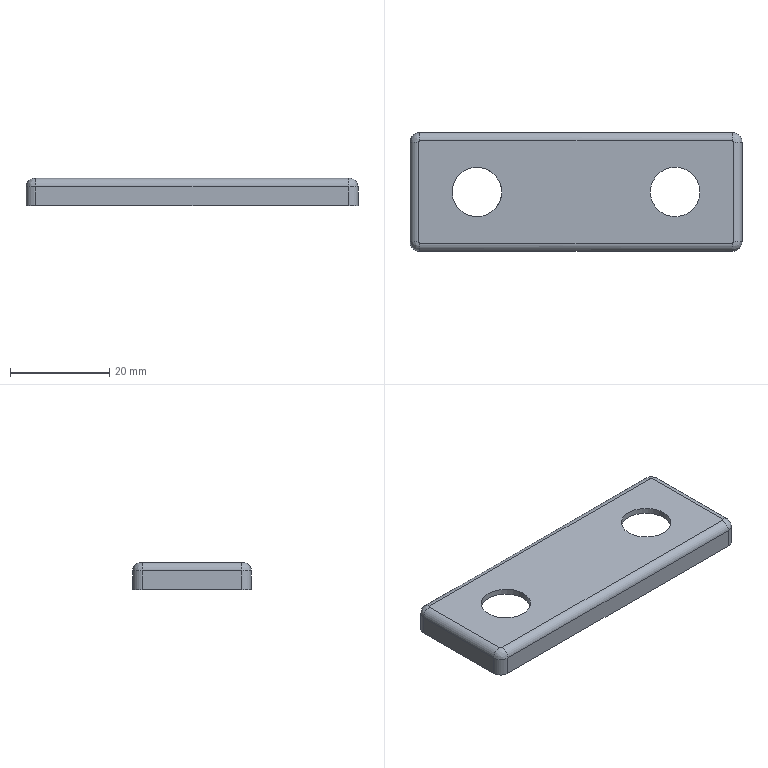Part | STEP file | FNA5401491 | 1 solid | 46 faces | box 67 x 24 x 5.5 mm | volume 2539 mm3 | spline 32 | cylinder 12 | plane 2 | commonest cylinder face diameters 1 x4 3.4 x4 10 x4